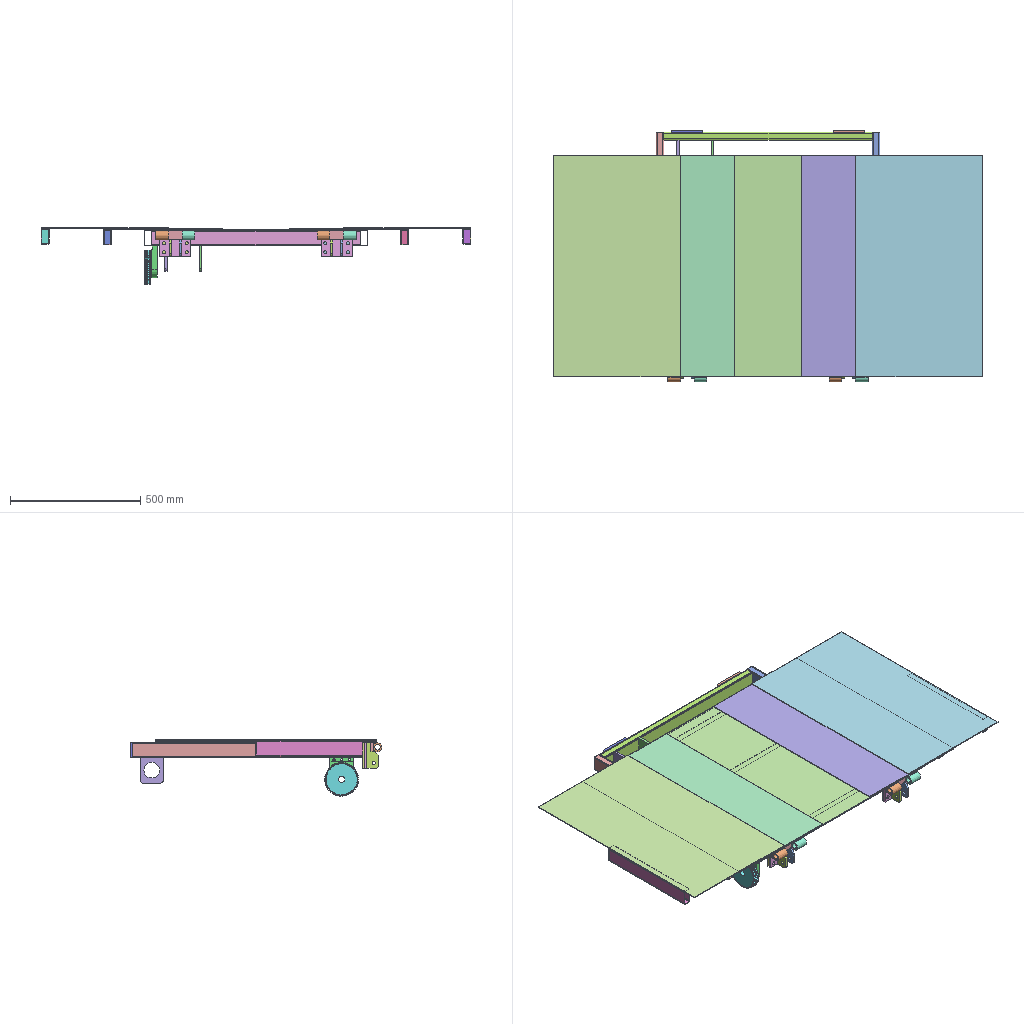Assembly | SolidWorks | 8 different items | 9 placed | box 1650 x 967 x 217 mm
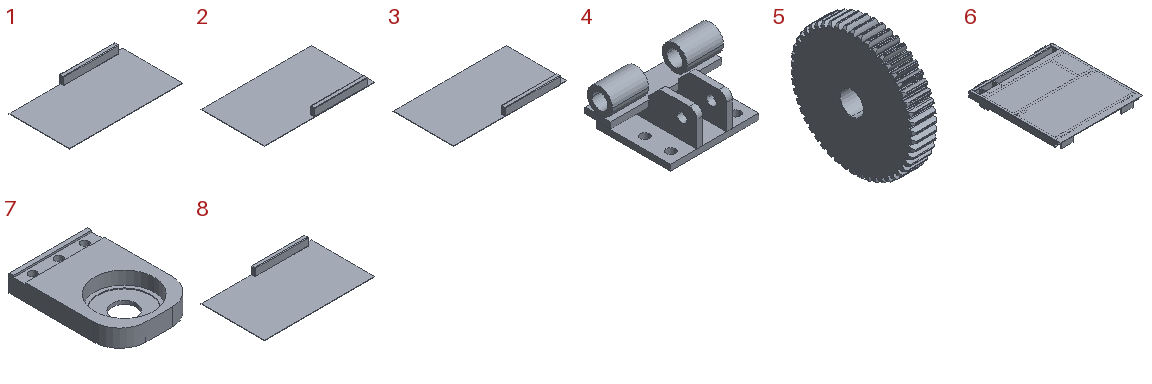Parts list (item | quantity | size | volume | features):
1 | x1 | 850 x 458 x 63 mm | 1296033 mm3 | features EndCap 1, Extrusion 1, WeldMemberFeat 1, WeldmentFeature 1
2 | x1 | 850 x 488 x 63 mm | 1385283 mm3 | features EndCap 1, Extrusion 1, WeldMemberFeat 1, WeldmentFeature 1
3 | x1 | 850 x 458 x 63 mm | 1296033 mm3 | features EndCap 1, Extrusion 1, WeldMemberFeat 1, WeldmentFeature 1
4 | x2 | 150 x 100 x 66.5 mm | 240667 mm3 | features ICE 6, Chamfer 2, Fillet 2, MoveCopyBody 2, Extrusion 1, MirrorSolid 1, MoveFace 1
5 | x1 | 45 x 129.796 x 130 mm | 311137 mm3 | features ICE 5, Chamfer 2, CirPattern 1, Extrusion 1, Fillet 1, RevCut 1
6 | x1 | 860 x 948 x 160 mm | 4527013 mm3 | features ICE 7, Split 3, WeldMemberFeat 3, LPattern 2, MirrorSolid 2, MoveFace 2, Fillet 1, WeldmentFeature 1
7 | x1 | 90 x 127.02 x 20 mm | 152136 mm3 | features ICE 4, MoveFace 2, Extrusion 1, Fillet 1, HoleWzd 1
8 | x1 | 850 x 488 x 63 mm | 1385283 mm3 | features EndCap 1, Extrusion 1, WeldMemberFeat 1, WeldmentFeature 1
Mates (type | each side: item.copy, entity, surface, feature):
Coincident | 6.1 face plane Mirror9 | 4.1 face plane Boss-Extrude1
Coincident | 6.1 face plane Mirror9 | 4.2 face plane Boss-Extrude1
Coincident | 6.1 face plane Boss-Extrude1 | 3.1 face plane Boss-Extrude1
Coincident | 6.1 face plane Split2 | 3.1 face plane Boss-Extrude1
Coincident | 3.1 face plane Boss-Extrude1 | 2.1 face plane Boss-Extrude1 | 2 times
Coincident | 6.1 face plane Boss-Extrude1 | 1.1 face plane Boss-Extrude1 | 2 times
Symmetric | 3.1 face plane Boss-Extrude1 | 1.1 face plane Boss-Extrude1 | assembly plane
Coincident | 1.1 face plane Boss-Extrude1 | 8.1 face plane Boss-Extrude1 | 2 times
Symmetric | 2.1 face plane Boss-Extrude1 | 8.1 face plane Boss-Extrude1 | assembly plane
LimitDistanceDim | 1.1 face plane Gb/6728-1986 rectangular hollow section 060 X 30 X 2(1) | 6.1 face plane Gb/6728-1986 rectangular hollow section 060 X 30 X 2(1)
LimitDistanceDim | 8.1 face plane Gb/6728-1986 rectangular hollow section 060 X 30 X 2(1) | 1.1 face plane Gb/6728-1986 rectangular hollow section 060 X 30 X 2(1)
Coincident | 6.1 face plane Gb/6728-1986 rectangular hollow section 060 X 30 X 2(1) | 7.1 face plane Boss-Extrude1
DistanceDim | 7.1 face plane Boss-Extrude1 | 6.1 face plane Gb/6728-1986 rectangular hollow section 060 X 30 X 2(1)
Concentric | 5.1 face cylinder Boss-Extrude1 | 7.1 face cylinder Cut-Extrude3
Coincident | 5.1 face plane Boss-Extrude2 | 7.1 face plane Boss-Extrude1